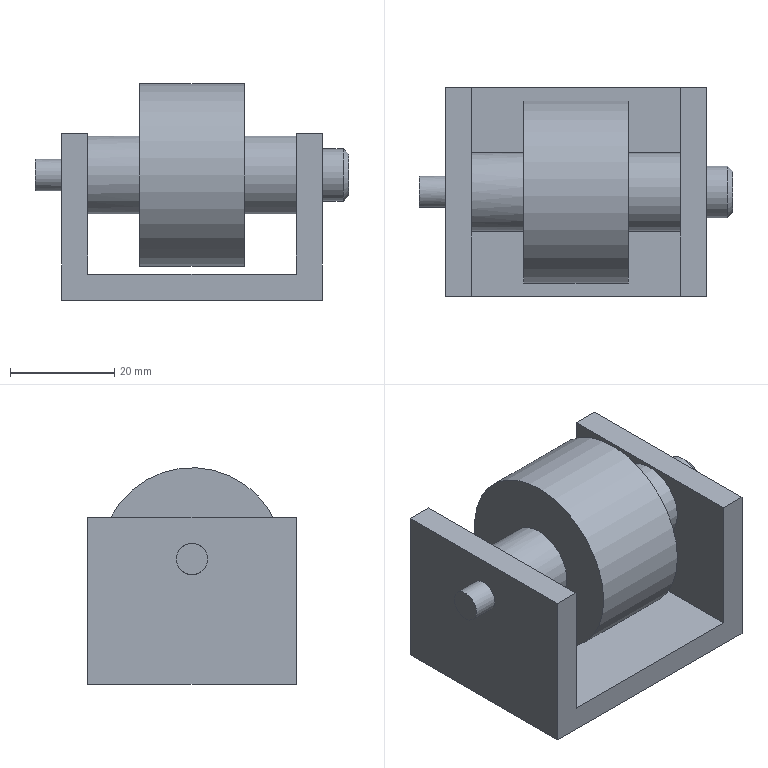Part | NX | features solid 2 | 1 solid | 20 faces | box 60 x 40 x 41.5 mm | volume 44096 mm3 | plane 14 | cylinder 5 | cone 1 | commonest cylinder face diameters 15 x2 6 x1 10 x1 35 x1
STEP:
#1=CARTESIAN_POINT('',(647.5,-180.,63.));
#2=VERTEX_POINT('',#1);
#3=CARTESIAN_POINT('',(647.5,-180.,59.));
#4=DIRECTION('',(1.,0.,0.));
#5=DIRECTION('',(0.,0.,1.));
#6=AXIS2_PLACEMENT_3D('',#3,#4,#5);
#7=CIRCLE('',#6,4.);
#8=EDGE_CURVE('',#2,#2,#7,.F.);
#9=ORIENTED_EDGE('',*,*,#8,.F.);
#10=EDGE_LOOP('',(#9));
#11=FACE_BOUND('',#10,.T.);
#12=CARTESIAN_POINT('',(647.5,-180.,59.));
#13=DIRECTION('',(-1.,0.,0.));
#14=DIRECTION('',(0.,0.,1.));
#15=AXIS2_PLACEMENT_3D('',#12,#13,#14);
#16=PLANE('',#15);
#17=ADVANCED_FACE('',(#11),#16,.F.);
#18=CARTESIAN_POINT('',(627.5,-197.5,59.));
#19=VERTEX_POINT('',#18);
#20=CARTESIAN_POINT('',(627.5,-180.,59.));
#21=DIRECTION('',(1.,0.,0.));
#22=DIRECTION('',(0.,-1.,0.));
#23=AXIS2_PLACEMENT_3D('',#20,#21,#22);
#24=CIRCLE('',#23,17.5);
#25=EDGE_CURVE('',#19,#19,#24,.T.);
#26=ORIENTED_EDGE('',*,*,#25,.F.);
#27=EDGE_LOOP('',(#26));
#28=FACE_BOUND('',#27,.T.);
#29=CARTESIAN_POINT('',(607.5,-197.5,59.));
#30=VERTEX_POINT('',#29);
#31=CARTESIAN_POINT('',(607.5,-180.,59.));
#32=DIRECTION('',(1.,0.,0.));
#33=DIRECTION('',(0.,-1.,0.));
#34=AXIS2_PLACEMENT_3D('',#31,#32,#33);
#35=CIRCLE('',#34,17.5);
#36=EDGE_CURVE('',#30,#30,#35,.T.);
#37=ORIENTED_EDGE('',*,*,#36,.T.);
#38=EDGE_LOOP('',(#37));
#39=FACE_BOUND('',#38,.T.);
#40=CARTESIAN_POINT('',(607.5,-180.,59.));
#41=DIRECTION('',(1.,0.,0.));
#42=DIRECTION('',(0.,0.,-1.));
#43=AXIS2_PLACEMENT_3D('',#40,#41,#42);
#44=CYLINDRICAL_SURFACE('',#43,17.5);
#45=ADVANCED_FACE('',(#28,#39),#44,.T.);
#46=CARTESIAN_POINT('',(646.5,-180.,64.));
#47=VERTEX_POINT('',#46);
#48=CARTESIAN_POINT('',(646.5,-180.,59.));
#49=DIRECTION('',(1.,0.,0.));
#50=DIRECTION('',(0.,0.,1.));
#51=AXIS2_PLACEMENT_3D('',#48,#49,#50);
#52=CIRCLE('',#51,5.);
#53=EDGE_CURVE('',#47,#47,#52,.T.);
#54=ORIENTED_EDGE('',*,*,#53,.T.);
#55=EDGE_LOOP('',(#54));
#56=FACE_BOUND('',#55,.T.);
#57=ORIENTED_EDGE('',*,*,#8,.T.);
#58=EDGE_LOOP('',(#57));
#59=FACE_BOUND('',#58,.T.);
#60=CARTESIAN_POINT('',(646.5,-180.,59.));
#61=DIRECTION('',(-1.,0.,0.));
#62=DIRECTION('',(0.,0.,1.));
#63=AXIS2_PLACEMENT_3D('',#60,#61,#62);
#64=CONICAL_SURFACE('',#63,5.,0.7854);
#65=ADVANCED_FACE('',(#56,#59),#64,.T.);
#66=CARTESIAN_POINT('',(587.5,-183.,59.));
#67=VERTEX_POINT('',#66);
#68=CARTESIAN_POINT('',(587.5,-180.,59.));
#69=DIRECTION('',(1.,0.,0.));
#70=DIRECTION('',(0.,-1.,0.));
#71=AXIS2_PLACEMENT_3D('',#68,#69,#70);
#72=CIRCLE('',#71,3.);
#73=EDGE_CURVE('',#67,#67,#72,.T.);
#74=ORIENTED_EDGE('',*,*,#73,.F.);
#75=EDGE_LOOP('',(#74));
#76=FACE_BOUND('',#75,.T.);
#77=CARTESIAN_POINT('',(587.5,-180.,59.));
#78=DIRECTION('',(-1.,0.,0.));
#79=DIRECTION('',(0.,0.,1.));
#80=AXIS2_PLACEMENT_3D('',#77,#78,#79);
#81=PLANE('',#80);
#82=ADVANCED_FACE('',(#76),#81,.T.);
#83=ORIENTED_EDGE('',*,*,#25,.T.);
#84=EDGE_LOOP('',(#83));
#85=FACE_BOUND('',#84,.T.);
#86=CARTESIAN_POINT('',(627.5,-187.5,59.));
#87=VERTEX_POINT('',#86);
#88=CARTESIAN_POINT('',(627.5,-180.,59.));
#89=DIRECTION('',(1.,0.,0.));
#90=DIRECTION('',(0.,-1.,0.));
#91=AXIS2_PLACEMENT_3D('',#88,#89,#90);
#92=CIRCLE('',#91,7.5);
#93=EDGE_CURVE('',#87,#87,#92,.T.);
#94=ORIENTED_EDGE('',*,*,#93,.F.);
#95=EDGE_LOOP('',(#94));
#96=FACE_BOUND('',#95,.T.);
#97=CARTESIAN_POINT('',(627.5,-180.,59.));
#98=DIRECTION('',(-1.,0.,0.));
#99=DIRECTION('',(0.,0.,1.));
#100=AXIS2_PLACEMENT_3D('',#97,#98,#99);
#101=PLANE('',#100);
#102=ADVANCED_FACE('',(#85,#96),#101,.F.);
#103=ORIENTED_EDGE('',*,*,#36,.F.);
#104=EDGE_LOOP('',(#103));
#105=FACE_BOUND('',#104,.T.);
#106=CARTESIAN_POINT('',(607.5,-187.5,59.));
#107=VERTEX_POINT('',#106);
#108=CARTESIAN_POINT('',(607.5,-180.,59.));
#109=DIRECTION('',(1.,0.,0.));
#110=DIRECTION('',(0.,-1.,0.));
#111=AXIS2_PLACEMENT_3D('',#108,#109,#110);
#112=CIRCLE('',#111,7.5);
#113=EDGE_CURVE('',#107,#107,#112,.T.);
#114=ORIENTED_EDGE('',*,*,#113,.T.);
#115=EDGE_LOOP('',(#114));
#116=FACE_BOUND('',#115,.T.);
#117=CARTESIAN_POINT('',(607.5,-180.,59.));
#118=DIRECTION('',(-1.,0.,0.));
#119=DIRECTION('',(0.,0.,1.));
#120=AXIS2_PLACEMENT_3D('',#117,#118,#119);
#121=PLANE('',#120);
#122=ADVANCED_FACE('',(#105,#116),#121,.T.);
#123=ORIENTED_EDGE('',*,*,#53,.F.);
#124=EDGE_LOOP('',(#123));
#125=FACE_BOUND('',#124,.T.);
#126=CARTESIAN_POINT('',(642.5,-180.,54.));
#127=VERTEX_POINT('',#126);
#128=CARTESIAN_POINT('',(642.5,-180.,59.));
#129=DIRECTION('',(-1.,0.,0.));
#130=DIRECTION('',(0.,0.,-1.));
#131=AXIS2_PLACEMENT_3D('',#128,#129,#130);
#132=CIRCLE('',#131,5.);
#133=EDGE_CURVE('',#127,#127,#132,.T.);
#134=ORIENTED_EDGE('',*,*,#133,.F.);
#135=EDGE_LOOP('',(#134));
#136=FACE_BOUND('',#135,.T.);
#137=CARTESIAN_POINT('',(647.5,-180.,59.));
#138=DIRECTION('',(-1.,0.,0.));
#139=DIRECTION('',(0.,0.,1.));
#140=AXIS2_PLACEMENT_3D('',#137,#138,#139);
#141=CYLINDRICAL_SURFACE('',#140,5.);
#142=ADVANCED_FACE('',(#125,#136),#141,.T.);
#143=CARTESIAN_POINT('',(592.5,-180.,62.));
#144=VERTEX_POINT('',#143);
#145=CARTESIAN_POINT('',(592.5,-180.,59.));
#146=DIRECTION('',(1.,0.,0.));
#147=DIRECTION('',(0.,0.,1.));
#148=AXIS2_PLACEMENT_3D('',#145,#146,#147);
#149=CIRCLE('',#148,3.);
#150=EDGE_CURVE('',#144,#144,#149,.F.);
#151=ORIENTED_EDGE('',*,*,#150,.T.);
#152=EDGE_LOOP('',(#151));
#153=FACE_BOUND('',#152,.T.);
#154=ORIENTED_EDGE('',*,*,#73,.T.);
#155=EDGE_LOOP('',(#154));
#156=FACE_BOUND('',#155,.T.);
#157=CARTESIAN_POINT('',(587.5,-180.,59.));
#158=DIRECTION('',(1.,0.,0.));
#159=DIRECTION('',(0.,0.,-1.));
#160=AXIS2_PLACEMENT_3D('',#157,#158,#159);
#161=CYLINDRICAL_SURFACE('',#160,3.);
#162=ADVANCED_FACE('',(#153,#156),#161,.T.);
#163=CARTESIAN_POINT('',(637.5,-187.5,59.));
#164=VERTEX_POINT('',#163);
#165=CARTESIAN_POINT('',(637.5,-180.,59.));
#166=DIRECTION('',(1.,0.,0.));
#167=DIRECTION('',(0.,-1.,0.));
#168=AXIS2_PLACEMENT_3D('',#165,#166,#167);
#169=CIRCLE('',#168,7.5);
#170=EDGE_CURVE('',#164,#164,#169,.T.);
#171=ORIENTED_EDGE('',*,*,#170,.F.);
#172=EDGE_LOOP('',(#171));
#173=FACE_BOUND('',#172,.T.);
#174=ORIENTED_EDGE('',*,*,#93,.T.);
#175=EDGE_LOOP('',(#174));
#176=FACE_BOUND('',#175,.T.);
#177=CARTESIAN_POINT('',(637.5,-180.,59.));
#178=DIRECTION('',(-1.,0.,0.));
#179=DIRECTION('',(0.,0.,1.));
#180=AXIS2_PLACEMENT_3D('',#177,#178,#179);
#181=CYLINDRICAL_SURFACE('',#180,7.5);
#182=ADVANCED_FACE('',(#173,#176),#181,.T.);
#183=CARTESIAN_POINT('',(637.5,-200.,40.));
#184=VERTEX_POINT('',#183);
#185=CARTESIAN_POINT('',(597.5,-200.,40.));
#186=VERTEX_POINT('',#185);
#187=CARTESIAN_POINT('',(642.5,-200.,40.));
#188=DIRECTION('',(-1.,0.,0.));
#189=VECTOR('',#188,1000.);
#190=LINE('',#187,#189);
#191=EDGE_CURVE('',#184,#186,#190,.T.);
#192=ORIENTED_EDGE('',*,*,#191,.T.);
#193=CARTESIAN_POINT('',(597.5,-200.,67.));
#194=VERTEX_POINT('',#193);
#195=CARTESIAN_POINT('',(597.5,-200.,35.));
#196=DIRECTION('',(0.,0.,1.));
#197=VECTOR('',#196,1000.);
#198=LINE('',#195,#197);
#199=EDGE_CURVE('',#186,#194,#198,.T.);
#200=ORIENTED_EDGE('',*,*,#199,.T.);
#201=CARTESIAN_POINT('',(592.5,-200.,67.));
#202=VERTEX_POINT('',#201);
#203=CARTESIAN_POINT('',(620.,-200.,67.));
#204=DIRECTION('',(-1.,0.,0.));
#205=VECTOR('',#204,1000.);
#206=LINE('',#203,#205);
#207=EDGE_CURVE('',#194,#202,#206,.T.);
#208=ORIENTED_EDGE('',*,*,#207,.T.);
#209=CARTESIAN_POINT('',(592.5,-200.,35.));
#210=VERTEX_POINT('',#209);
#211=CARTESIAN_POINT('',(592.5,-200.,35.));
#212=DIRECTION('',(0.,0.,1.));
#213=VECTOR('',#212,1000.);
#214=LINE('',#211,#213);
#215=EDGE_CURVE('',#210,#202,#214,.T.);
#216=ORIENTED_EDGE('',*,*,#215,.F.);
#217=CARTESIAN_POINT('',(642.5,-200.,35.));
#218=VERTEX_POINT('',#217);
#219=CARTESIAN_POINT('',(642.5,-200.,35.));
#220=DIRECTION('',(-1.,0.,0.));
#221=VECTOR('',#220,1000.);
#222=LINE('',#219,#221);
#223=EDGE_CURVE('',#218,#210,#222,.T.);
#224=ORIENTED_EDGE('',*,*,#223,.F.);
#225=CARTESIAN_POINT('',(642.5,-200.,67.));
#226=VERTEX_POINT('',#225);
#227=CARTESIAN_POINT('',(642.5,-200.,67.));
#228=DIRECTION('',(0.,0.,-1.));
#229=VECTOR('',#228,1000.);
#230=LINE('',#227,#229);
#231=EDGE_CURVE('',#226,#218,#230,.T.);
#232=ORIENTED_EDGE('',*,*,#231,.F.);
#233=CARTESIAN_POINT('',(637.5,-200.,67.));
#234=VERTEX_POINT('',#233);
#235=CARTESIAN_POINT('',(620.,-200.,67.));
#236=DIRECTION('',(1.,0.,0.));
#237=VECTOR('',#236,1000.);
#238=LINE('',#235,#237);
#239=EDGE_CURVE('',#226,#234,#238,.F.);
#240=ORIENTED_EDGE('',*,*,#239,.T.);
#241=CARTESIAN_POINT('',(637.5,-200.,67.));
#242=DIRECTION('',(0.,0.,-1.));
#243=VECTOR('',#242,1000.);
#244=LINE('',#241,#243);
#245=EDGE_CURVE('',#234,#184,#244,.T.);
#246=ORIENTED_EDGE('',*,*,#245,.T.);
#247=EDGE_LOOP('',(#192,#200,#208,#216,#224,#232,#240,#246));
#248=FACE_BOUND('',#247,.T.);
#249=CARTESIAN_POINT('',(620.,-200.,55.62));
#250=DIRECTION('',(0.,1.,0.));
#251=DIRECTION('',(0.,0.,1.));
#252=AXIS2_PLACEMENT_3D('',#249,#250,#251);
#253=PLANE('',#252);
#254=ADVANCED_FACE('',(#248),#253,.F.);
#255=ORIENTED_EDGE('',*,*,#113,.F.);
#256=EDGE_LOOP('',(#255));
#257=FACE_BOUND('',#256,.T.);
#258=CARTESIAN_POINT('',(597.5,-180.,66.5));
#259=VERTEX_POINT('',#258);
#260=CARTESIAN_POINT('',(597.5,-180.,59.));
#261=DIRECTION('',(1.,0.,0.));
#262=DIRECTION('',(0.,0.,1.));
#263=AXIS2_PLACEMENT_3D('',#260,#261,#262);
#264=CIRCLE('',#263,7.5);
#265=EDGE_CURVE('',#259,#259,#264,.F.);
#266=ORIENTED_EDGE('',*,*,#265,.F.);
#267=EDGE_LOOP('',(#266));
#268=FACE_BOUND('',#267,.T.);
#269=CARTESIAN_POINT('',(597.5,-180.,59.));
#270=DIRECTION('',(1.,0.,0.));
#271=DIRECTION('',(0.,0.,-1.));
#272=AXIS2_PLACEMENT_3D('',#269,#270,#271);
#273=CYLINDRICAL_SURFACE('',#272,7.5);
#274=ADVANCED_FACE('',(#257,#268),#273,.T.);
#275=ORIENTED_EDGE('',*,*,#265,.T.);
#276=EDGE_LOOP('',(#275));
#277=FACE_BOUND('',#276,.T.);
#278=CARTESIAN_POINT('',(597.5,-160.,40.));
#279=VERTEX_POINT('',#278);
#280=CARTESIAN_POINT('',(597.5,-160.,67.));
#281=VERTEX_POINT('',#280);
#282=CARTESIAN_POINT('',(597.5,-160.,35.));
#283=DIRECTION('',(0.,0.,1.));
#284=VECTOR('',#283,1000.);
#285=LINE('',#282,#284);
#286=EDGE_CURVE('',#279,#281,#285,.T.);
#287=ORIENTED_EDGE('',*,*,#286,.T.);
#288=CARTESIAN_POINT('',(597.5,-123.,67.));
#289=DIRECTION('',(0.,-1.,0.));
#290=VECTOR('',#289,1000.);
#291=LINE('',#288,#290);
#292=EDGE_CURVE('',#281,#194,#291,.T.);
#293=ORIENTED_EDGE('',*,*,#292,.T.);
#294=ORIENTED_EDGE('',*,*,#199,.F.);
#295=CARTESIAN_POINT('',(597.5,-123.,40.));
#296=DIRECTION('',(0.,-1.,0.));
#297=VECTOR('',#296,1000.);
#298=LINE('',#295,#297);
#299=EDGE_CURVE('',#279,#186,#298,.T.);
#300=ORIENTED_EDGE('',*,*,#299,.F.);
#301=EDGE_LOOP('',(#287,#293,#294,#300));
#302=FACE_BOUND('',#301,.T.);
#303=CARTESIAN_POINT('',(597.5,-123.,35.));
#304=DIRECTION('',(-1.,0.,0.));
#305=DIRECTION('',(0.,0.,1.));
#306=AXIS2_PLACEMENT_3D('',#303,#304,#305);
#307=PLANE('',#306);
#308=ADVANCED_FACE('',(#277,#302),#307,.F.);
#309=ORIENTED_EDGE('',*,*,#150,.F.);
#310=EDGE_LOOP('',(#309));
#311=FACE_BOUND('',#310,.T.);
#312=CARTESIAN_POINT('',(592.5,-160.,35.));
#313=VERTEX_POINT('',#312);
#314=CARTESIAN_POINT('',(592.5,-123.,35.));
#315=DIRECTION('',(0.,-1.,0.));
#316=VECTOR('',#315,1000.);
#317=LINE('',#314,#316);
#318=EDGE_CURVE('',#313,#210,#317,.T.);
#319=ORIENTED_EDGE('',*,*,#318,.T.);
#320=ORIENTED_EDGE('',*,*,#215,.T.);
#321=CARTESIAN_POINT('',(592.5,-160.,67.));
#322=VERTEX_POINT('',#321);
#323=CARTESIAN_POINT('',(592.5,-123.,67.));
#324=DIRECTION('',(0.,-1.,0.));
#325=VECTOR('',#324,1000.);
#326=LINE('',#323,#325);
#327=EDGE_CURVE('',#322,#202,#326,.T.);
#328=ORIENTED_EDGE('',*,*,#327,.F.);
#329=CARTESIAN_POINT('',(592.5,-160.,35.));
#330=DIRECTION('',(0.,0.,1.));
#331=VECTOR('',#330,1000.);
#332=LINE('',#329,#331);
#333=EDGE_CURVE('',#313,#322,#332,.T.);
#334=ORIENTED_EDGE('',*,*,#333,.F.);
#335=EDGE_LOOP('',(#319,#320,#328,#334));
#336=FACE_BOUND('',#335,.T.);
#337=CARTESIAN_POINT('',(592.5,-123.,35.));
#338=DIRECTION('',(-1.,0.,0.));
#339=DIRECTION('',(0.,0.,1.));
#340=AXIS2_PLACEMENT_3D('',#337,#338,#339);
#341=PLANE('',#340);
#342=ADVANCED_FACE('',(#311,#336),#341,.T.);
#343=ORIENTED_EDGE('',*,*,#170,.T.);
#344=EDGE_LOOP('',(#343));
#345=FACE_BOUND('',#344,.T.);
#346=CARTESIAN_POINT('',(637.5,-160.,67.));
#347=VERTEX_POINT('',#346);
#348=CARTESIAN_POINT('',(637.5,-160.,40.));
#349=VERTEX_POINT('',#348);
#350=CARTESIAN_POINT('',(637.5,-160.,67.));
#351=DIRECTION('',(0.,0.,-1.));
#352=VECTOR('',#351,1000.);
#353=LINE('',#350,#352);
#354=EDGE_CURVE('',#347,#349,#353,.T.);
#355=ORIENTED_EDGE('',*,*,#354,.T.);
#356=CARTESIAN_POINT('',(637.5,-123.,40.));
#357=DIRECTION('',(0.,-1.,0.));
#358=VECTOR('',#357,1000.);
#359=LINE('',#356,#358);
#360=EDGE_CURVE('',#349,#184,#359,.T.);
#361=ORIENTED_EDGE('',*,*,#360,.T.);
#362=ORIENTED_EDGE('',*,*,#245,.F.);
#363=CARTESIAN_POINT('',(637.5,-123.,67.));
#364=DIRECTION('',(0.,-1.,0.));
#365=VECTOR('',#364,1000.);
#366=LINE('',#363,#365);
#367=EDGE_CURVE('',#347,#234,#366,.T.);
#368=ORIENTED_EDGE('',*,*,#367,.F.);
#369=EDGE_LOOP('',(#355,#361,#362,#368));
#370=FACE_BOUND('',#369,.T.);
#371=CARTESIAN_POINT('',(637.5,-123.,67.));
#372=DIRECTION('',(1.,0.,0.));
#373=DIRECTION('',(0.,0.,-1.));
#374=AXIS2_PLACEMENT_3D('',#371,#372,#373);
#375=PLANE('',#374);
#376=ADVANCED_FACE('',(#345,#370),#375,.F.);
#377=ORIENTED_EDGE('',*,*,#133,.T.);
#378=EDGE_LOOP('',(#377));
#379=FACE_BOUND('',#378,.T.);
#380=CARTESIAN_POINT('',(642.5,-160.,67.));
#381=VERTEX_POINT('',#380);
#382=CARTESIAN_POINT('',(642.5,-123.,67.));
#383=DIRECTION('',(0.,-1.,0.));
#384=VECTOR('',#383,1000.);
#385=LINE('',#382,#384);
#386=EDGE_CURVE('',#381,#226,#385,.T.);
#387=ORIENTED_EDGE('',*,*,#386,.T.);
#388=ORIENTED_EDGE('',*,*,#231,.T.);
#389=CARTESIAN_POINT('',(642.5,-160.,35.));
#390=VERTEX_POINT('',#389);
#391=CARTESIAN_POINT('',(642.5,-123.,35.));
#392=DIRECTION('',(0.,-1.,0.));
#393=VECTOR('',#392,1000.);
#394=LINE('',#391,#393);
#395=EDGE_CURVE('',#390,#218,#394,.T.);
#396=ORIENTED_EDGE('',*,*,#395,.F.);
#397=CARTESIAN_POINT('',(642.5,-160.,67.));
#398=DIRECTION('',(0.,0.,-1.));
#399=VECTOR('',#398,1000.);
#400=LINE('',#397,#399);
#401=EDGE_CURVE('',#381,#390,#400,.T.);
#402=ORIENTED_EDGE('',*,*,#401,.F.);
#403=EDGE_LOOP('',(#387,#388,#396,#402));
#404=FACE_BOUND('',#403,.T.);
#405=CARTESIAN_POINT('',(642.5,-123.,67.));
#406=DIRECTION('',(1.,0.,0.));
#407=DIRECTION('',(0.,0.,-1.));
#408=AXIS2_PLACEMENT_3D('',#405,#406,#407);
#409=PLANE('',#408);
#410=ADVANCED_FACE('',(#379,#404),#409,.T.);
#411=ORIENTED_EDGE('',*,*,#367,.T.);
#412=ORIENTED_EDGE('',*,*,#239,.F.);
#413=ORIENTED_EDGE('',*,*,#386,.F.);
#414=CARTESIAN_POINT('',(642.5,-160.,67.));
#415=DIRECTION('',(-1.,0.,0.));
#416=VECTOR('',#415,1000.);
#417=LINE('',#414,#416);
#418=EDGE_CURVE('',#347,#381,#417,.F.);
#419=ORIENTED_EDGE('',*,*,#418,.F.);
#420=EDGE_LOOP('',(#411,#412,#413,#419));
#421=FACE_BOUND('',#420,.T.);
#422=CARTESIAN_POINT('',(642.5,-123.,67.));
#423=DIRECTION('',(0.,0.,-1.));
#424=DIRECTION('',(0.,-1.,0.));
#425=AXIS2_PLACEMENT_3D('',#422,#423,#424);
#426=PLANE('',#425);
#427=ADVANCED_FACE('',(#421),#426,.F.);
#428=ORIENTED_EDGE('',*,*,#395,.T.);
#429=ORIENTED_EDGE('',*,*,#223,.T.);
#430=ORIENTED_EDGE('',*,*,#318,.F.);
#431=CARTESIAN_POINT('',(642.5,-160.,35.));
#432=DIRECTION('',(-1.,0.,0.));
#433=VECTOR('',#432,1000.);
#434=LINE('',#431,#433);
#435=EDGE_CURVE('',#390,#313,#434,.T.);
#436=ORIENTED_EDGE('',*,*,#435,.F.);
#437=EDGE_LOOP('',(#428,#429,#430,#436));
#438=FACE_BOUND('',#437,.T.);
#439=CARTESIAN_POINT('',(642.5,-123.,35.));
#440=DIRECTION('',(0.,0.,-1.));
#441=DIRECTION('',(0.,1.,0.));
#442=AXIS2_PLACEMENT_3D('',#439,#440,#441);
#443=PLANE('',#442);
#444=ADVANCED_FACE('',(#438),#443,.T.);
#445=ORIENTED_EDGE('',*,*,#327,.T.);
#446=ORIENTED_EDGE('',*,*,#207,.F.);
#447=ORIENTED_EDGE('',*,*,#292,.F.);
#448=CARTESIAN_POINT('',(592.5,-160.,67.));
#449=DIRECTION('',(1.,0.,0.));
#450=VECTOR('',#449,1000.);
#451=LINE('',#448,#450);
#452=EDGE_CURVE('',#322,#281,#451,.T.);
#453=ORIENTED_EDGE('',*,*,#452,.F.);
#454=EDGE_LOOP('',(#445,#446,#447,#453));
#455=FACE_BOUND('',#454,.T.);
#456=CARTESIAN_POINT('',(592.5,-123.,67.));
#457=DIRECTION('',(0.,0.,1.));
#458=DIRECTION('',(0.,-1.,0.));
#459=AXIS2_PLACEMENT_3D('',#456,#457,#458);
#460=PLANE('',#459);
#461=ADVANCED_FACE('',(#455),#460,.T.);
#462=CARTESIAN_POINT('',(642.5,-160.,40.));
#463=DIRECTION('',(-1.,0.,0.));
#464=VECTOR('',#463,1000.);
#465=LINE('',#462,#464);
#466=EDGE_CURVE('',#349,#279,#465,.T.);
#467=ORIENTED_EDGE('',*,*,#466,.T.);
#468=ORIENTED_EDGE('',*,*,#299,.T.);
#469=ORIENTED_EDGE('',*,*,#191,.F.);
#470=ORIENTED_EDGE('',*,*,#360,.F.);
#471=EDGE_LOOP('',(#467,#468,#469,#470));
#472=FACE_BOUND('',#471,.T.);
#473=CARTESIAN_POINT('',(642.5,-123.,40.));
#474=DIRECTION('',(0.,0.,-1.));
#475=DIRECTION('',(0.,1.,0.));
#476=AXIS2_PLACEMENT_3D('',#473,#474,#475);
#477=PLANE('',#476);
#478=ADVANCED_FACE('',(#472),#477,.F.);
#479=ORIENTED_EDGE('',*,*,#452,.T.);
#480=ORIENTED_EDGE('',*,*,#286,.F.);
#481=ORIENTED_EDGE('',*,*,#466,.F.);
#482=ORIENTED_EDGE('',*,*,#354,.F.);
#483=ORIENTED_EDGE('',*,*,#418,.T.);
#484=ORIENTED_EDGE('',*,*,#401,.T.);
#485=ORIENTED_EDGE('',*,*,#435,.T.);
#486=ORIENTED_EDGE('',*,*,#333,.T.);
#487=EDGE_LOOP('',(#479,#480,#481,#482,#483,#484,#485,#486));
#488=FACE_BOUND('',#487,.T.);
#489=CARTESIAN_POINT('',(617.5,-160.,48.5));
#490=DIRECTION('',(0.,1.,0.));
#491=DIRECTION('',(0.,0.,1.));
#492=AXIS2_PLACEMENT_3D('',#489,#490,#491);
#493=PLANE('',#492);
#494=ADVANCED_FACE('',(#488),#493,.T.);
#495=CLOSED_SHELL('',(#17,#45,#65,#82,#102,#122,#142,#162,#182,#254,#274,#308,#342,#376,#410,#427,#444,#461,#478,#494));
#496=MANIFOLD_SOLID_BREP('',#495);
#497=(LENGTH_UNIT()NAMED_UNIT(*)SI_UNIT(.MILLI.,.METRE.));
#498=UNCERTAINTY_MEASURE_WITH_UNIT(LENGTH_MEASURE(0.00001),#497,'','');
#499=(NAMED_UNIT(*)PLANE_ANGLE_UNIT()SI_UNIT($,.RADIAN.));
#500=(NAMED_UNIT(*)SI_UNIT($,.STERADIAN.)SOLID_ANGLE_UNIT());
#501=(GEOMETRIC_REPRESENTATION_CONTEXT(3)GLOBAL_UNCERTAINTY_ASSIGNED_CONTEXT((#498))GLOBAL_UNIT_ASSIGNED_CONTEXT((#497,#499,#500))REPRESENTATION_CONTEXT('',''));
#502=ADVANCED_BREP_SHAPE_REPRESENTATION('',(#496),#501);